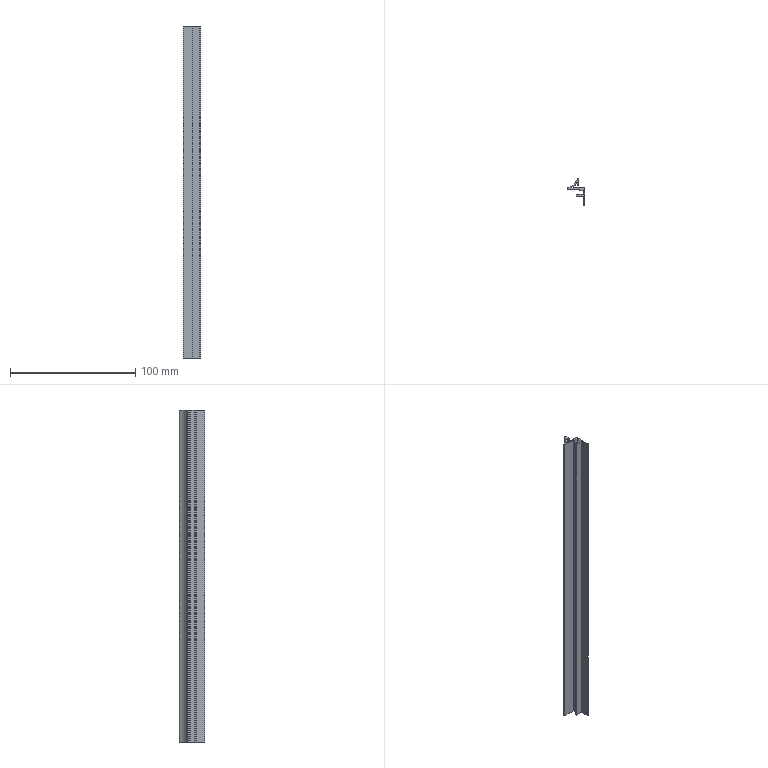Part | SolidWorks | features MoveFace 2, BaseBody 1, ICE 1 | 1 solid | 27 faces | box 14 x 20.3 x 265 mm | volume 13493 mm3 | plane 20 | cylinder 7 | commonest cylinder face diameters 0.387 x2 0.8 x2 0.4 x1 20 x1 22 x1
STEP:
#1=CARTESIAN_POINT('',(-5.304,-0.625,320.));
#2=VERTEX_POINT('',#1);
#3=CARTESIAN_POINT('',(-5.449,-0.8125,320.));
#4=VERTEX_POINT('',#3);
#5=CARTESIAN_POINT('',(-5.255,-0.8125,320.));
#6=DIRECTION('',(0.,0.,1.));
#7=DIRECTION('',(-1.,0.,0.));
#8=AXIS2_PLACEMENT_3D('',#5,#6,#7);
#9=CIRCLE('',#8,0.1937);
#10=EDGE_CURVE('',#2,#4,#9,.T.);
#11=ORIENTED_EDGE('',*,*,#10,.T.);
#12=CARTESIAN_POINT('',(-5.449,-0.8125,55.));
#13=VERTEX_POINT('',#12);
#14=CARTESIAN_POINT('',(-5.449,-0.8125,230.));
#15=DIRECTION('',(0.,0.,-1.));
#16=VECTOR('',#15,1000.);
#17=LINE('',#14,#16);
#18=EDGE_CURVE('',#4,#13,#17,.T.);
#19=ORIENTED_EDGE('',*,*,#18,.T.);
#20=CARTESIAN_POINT('',(-5.304,-0.625,55.));
#21=VERTEX_POINT('',#20);
#22=CARTESIAN_POINT('',(-5.255,-0.8125,55.));
#23=DIRECTION('',(0.,0.,-1.));
#24=DIRECTION('',(1.,0.,0.));
#25=AXIS2_PLACEMENT_3D('',#22,#23,#24);
#26=CIRCLE('',#25,0.1937);
#27=EDGE_CURVE('',#13,#21,#26,.T.);
#28=ORIENTED_EDGE('',*,*,#27,.T.);
#29=CARTESIAN_POINT('',(-5.304,-0.625,230.));
#30=DIRECTION('',(0.,0.,-1.));
#31=VECTOR('',#30,1000.);
#32=LINE('',#29,#31);
#33=EDGE_CURVE('',#2,#21,#32,.T.);
#34=ORIENTED_EDGE('',*,*,#33,.F.);
#35=EDGE_LOOP('',(#11,#19,#28,#34));
#36=FACE_OUTER_BOUND('',#35,.T.);
#37=CARTESIAN_POINT('',(-5.255,-0.8125,230.));
#38=DIRECTION('',(0.,0.,-1.));
#39=DIRECTION('',(-1.,0.,0.));
#40=AXIS2_PLACEMENT_3D('',#37,#38,#39);
#41=CYLINDRICAL_SURFACE('',#40,0.1937);
#42=ADVANCED_FACE('',(#36),#41,.F.);
#43=CARTESIAN_POINT('',(5.,-1.,55.));
#44=VERTEX_POINT('',#43);
#45=CARTESIAN_POINT('',(5.,-14.3,55.));
#46=VERTEX_POINT('',#45);
#47=CARTESIAN_POINT('',(5.,29.623,55.));
#48=DIRECTION('',(0.,-1.,0.));
#49=VECTOR('',#48,1000.);
#50=LINE('',#47,#49);
#51=EDGE_CURVE('',#44,#46,#50,.T.);
#52=ORIENTED_EDGE('',*,*,#51,.F.);
#53=CARTESIAN_POINT('',(5.,-1.,320.));
#54=VERTEX_POINT('',#53);
#55=CARTESIAN_POINT('',(5.,-1.,230.));
#56=DIRECTION('',(0.,0.,-1.));
#57=VECTOR('',#56,1000.);
#58=LINE('',#55,#57);
#59=EDGE_CURVE('',#54,#44,#58,.T.);
#60=ORIENTED_EDGE('',*,*,#59,.F.);
#61=CARTESIAN_POINT('',(5.,-14.3,320.));
#62=VERTEX_POINT('',#61);
#63=CARTESIAN_POINT('',(5.,29.623,320.));
#64=DIRECTION('',(0.,1.,0.));
#65=VECTOR('',#64,1000.);
#66=LINE('',#63,#65);
#67=EDGE_CURVE('',#62,#54,#66,.T.);
#68=ORIENTED_EDGE('',*,*,#67,.F.);
#69=CARTESIAN_POINT('',(5.,-14.3,230.));
#70=DIRECTION('',(0.,0.,1.));
#71=VECTOR('',#70,1000.);
#72=LINE('',#69,#71);
#73=EDGE_CURVE('',#46,#62,#72,.T.);
#74=ORIENTED_EDGE('',*,*,#73,.F.);
#75=EDGE_LOOP('',(#52,#60,#68,#74));
#76=FACE_OUTER_BOUND('',#75,.T.);
#77=CARTESIAN_POINT('',(5.,-14.3,230.));
#78=DIRECTION('',(-1.,0.,0.));
#79=DIRECTION('',(0.,0.,1.));
#80=AXIS2_PLACEMENT_3D('',#77,#78,#79);
#81=PLANE('',#80);
#82=ADVANCED_FACE('',(#76),#81,.F.);
#83=CARTESIAN_POINT('',(-9.,-2.,55.));
#84=VERTEX_POINT('',#83);
#85=CARTESIAN_POINT('',(-9.,-2.,320.));
#86=VERTEX_POINT('',#85);
#87=CARTESIAN_POINT('',(-9.,-2.,230.));
#88=DIRECTION('',(0.,0.,1.));
#89=VECTOR('',#88,1000.);
#90=LINE('',#87,#89);
#91=EDGE_CURVE('',#84,#86,#90,.T.);
#92=ORIENTED_EDGE('',*,*,#91,.F.);
#93=CARTESIAN_POINT('',(0.9,-2.,55.));
#94=VERTEX_POINT('',#93);
#95=CARTESIAN_POINT('',(5.,-2.,55.));
#96=DIRECTION('',(-1.,0.,0.));
#97=VECTOR('',#96,1000.);
#98=LINE('',#95,#97);
#99=EDGE_CURVE('',#94,#84,#98,.T.);
#100=ORIENTED_EDGE('',*,*,#99,.F.);
#101=CARTESIAN_POINT('',(0.9,-2.,320.));
#102=VERTEX_POINT('',#101);
#103=CARTESIAN_POINT('',(0.9,-2.,230.));
#104=DIRECTION('',(0.,0.,-1.));
#105=VECTOR('',#104,1000.);
#106=LINE('',#103,#105);
#107=EDGE_CURVE('',#102,#94,#106,.T.);
#108=ORIENTED_EDGE('',*,*,#107,.F.);
#109=CARTESIAN_POINT('',(5.,-2.,320.));
#110=DIRECTION('',(1.,0.,0.));
#111=VECTOR('',#110,1000.);
#112=LINE('',#109,#111);
#113=EDGE_CURVE('',#86,#102,#112,.T.);
#114=ORIENTED_EDGE('',*,*,#113,.F.);
#115=EDGE_LOOP('',(#92,#100,#108,#114));
#116=FACE_OUTER_BOUND('',#115,.T.);
#117=CARTESIAN_POINT('',(-9.,-2.,230.));
#118=DIRECTION('',(0.,1.,0.));
#119=DIRECTION('',(0.,0.,1.));
#120=AXIS2_PLACEMENT_3D('',#117,#118,#119);
#121=PLANE('',#120);
#122=ADVANCED_FACE('',(#116),#121,.F.);
#123=CARTESIAN_POINT('',(4.,-6.,320.));
#124=VERTEX_POINT('',#123);
#125=CARTESIAN_POINT('',(4.,-3.,320.));
#126=VERTEX_POINT('',#125);
#127=CARTESIAN_POINT('',(4.,-3.,320.));
#128=DIRECTION('',(0.,1.,0.));
#129=VECTOR('',#128,1000.);
#130=LINE('',#127,#129);
#131=EDGE_CURVE('',#124,#126,#130,.T.);
#132=ORIENTED_EDGE('',*,*,#131,.F.);
#133=CARTESIAN_POINT('',(1.,-6.,320.));
#134=VERTEX_POINT('',#133);
#135=CARTESIAN_POINT('',(4.,-6.,320.));
#136=DIRECTION('',(1.,0.,0.));
#137=VECTOR('',#136,1000.);
#138=LINE('',#135,#137);
#139=EDGE_CURVE('',#134,#124,#138,.T.);
#140=ORIENTED_EDGE('',*,*,#139,.F.);
#141=CARTESIAN_POINT('',(1.,-6.7,320.));
#142=VERTEX_POINT('',#141);
#143=CARTESIAN_POINT('',(1.,29.623,320.));
#144=DIRECTION('',(0.,-1.,0.));
#145=VECTOR('',#144,1000.);
#146=LINE('',#143,#145);
#147=EDGE_CURVE('',#134,#142,#146,.T.);
#148=ORIENTED_EDGE('',*,*,#147,.T.);
#149=CARTESIAN_POINT('',(-1.7,-6.7,320.));
#150=VERTEX_POINT('',#149);
#151=CARTESIAN_POINT('',(1.,-6.7,320.));
#152=DIRECTION('',(1.,0.,0.));
#153=VECTOR('',#152,1000.);
#154=LINE('',#151,#153);
#155=EDGE_CURVE('',#150,#142,#154,.T.);
#156=ORIENTED_EDGE('',*,*,#155,.F.);
#157=CARTESIAN_POINT('',(-1.7,-7.7,320.));
#158=VERTEX_POINT('',#157);
#159=CARTESIAN_POINT('',(-1.7,29.623,320.));
#160=DIRECTION('',(0.,-1.,0.));
#161=VECTOR('',#160,1000.);
#162=LINE('',#159,#161);
#163=EDGE_CURVE('',#150,#158,#162,.T.);
#164=ORIENTED_EDGE('',*,*,#163,.T.);
#165=CARTESIAN_POINT('',(4.,-7.7,320.));
#166=VERTEX_POINT('',#165);
#167=CARTESIAN_POINT('',(-1.7,-7.7,320.));
#168=DIRECTION('',(-1.,0.,0.));
#169=VECTOR('',#168,1000.);
#170=LINE('',#167,#169);
#171=EDGE_CURVE('',#166,#158,#170,.T.);
#172=ORIENTED_EDGE('',*,*,#171,.F.);
#173=CARTESIAN_POINT('',(4.,-14.3,320.));
#174=VERTEX_POINT('',#173);
#175=CARTESIAN_POINT('',(4.,-7.7,320.));
#176=DIRECTION('',(0.,1.,0.));
#177=VECTOR('',#176,1000.);
#178=LINE('',#175,#177);
#179=EDGE_CURVE('',#174,#166,#178,.T.);
#180=ORIENTED_EDGE('',*,*,#179,.F.);
#181=CARTESIAN_POINT('',(4.,-14.3,320.));
#182=DIRECTION('',(-1.,0.,0.));
#183=VECTOR('',#182,1000.);
#184=LINE('',#181,#183);
#185=EDGE_CURVE('',#62,#174,#184,.T.);
#186=ORIENTED_EDGE('',*,*,#185,.F.);
#187=ORIENTED_EDGE('',*,*,#67,.T.);
#188=CARTESIAN_POINT('',(-5.207,-1.,320.));
#189=VERTEX_POINT('',#188);
#190=CARTESIAN_POINT('',(5.,-1.,320.));
#191=DIRECTION('',(1.,0.,0.));
#192=VECTOR('',#191,1000.);
#193=LINE('',#190,#192);
#194=EDGE_CURVE('',#189,#54,#193,.T.);
#195=ORIENTED_EDGE('',*,*,#194,.F.);
#196=CARTESIAN_POINT('',(-5.255,-0.8125,320.));
#197=DIRECTION('',(0.,0.,1.));
#198=DIRECTION('',(-1.,0.,0.));
#199=AXIS2_PLACEMENT_3D('',#196,#197,#198);
#200=CIRCLE('',#199,0.1937);
#201=EDGE_CURVE('',#4,#189,#200,.T.);
#202=ORIENTED_EDGE('',*,*,#201,.F.);
#203=ORIENTED_EDGE('',*,*,#10,.F.);
#204=CARTESIAN_POINT('',(-1.368,3.063,320.));
#205=VERTEX_POINT('',#204);
#206=CARTESIAN_POINT('',(-10.628,9.,320.));
#207=DIRECTION('',(0.,0.,1.));
#208=DIRECTION('',(-1.,0.,0.));
#209=AXIS2_PLACEMENT_3D('',#206,#207,#208);
#210=CIRCLE('',#209,11.);
#211=EDGE_CURVE('',#2,#205,#210,.T.);
#212=ORIENTED_EDGE('',*,*,#211,.T.);
#213=CARTESIAN_POINT('',(-1.,2.955,320.));
#214=VERTEX_POINT('',#213);
#215=CARTESIAN_POINT('',(-1.2,2.955,320.));
#216=DIRECTION('',(0.,0.,1.));
#217=DIRECTION('',(-1.,0.,0.));
#218=AXIS2_PLACEMENT_3D('',#215,#216,#217);
#219=CIRCLE('',#218,0.2);
#220=EDGE_CURVE('',#214,#205,#219,.T.);
#221=ORIENTED_EDGE('',*,*,#220,.F.);
#222=CARTESIAN_POINT('',(-1.,1.5,320.));
#223=VERTEX_POINT('',#222);
#224=CARTESIAN_POINT('',(-1.,2.955,320.));
#225=DIRECTION('',(0.,1.,0.));
#226=VECTOR('',#225,1000.);
#227=LINE('',#224,#226);
#228=EDGE_CURVE('',#223,#214,#227,.T.);
#229=ORIENTED_EDGE('',*,*,#228,.F.);
#230=CARTESIAN_POINT('',(0.,1.5,320.));
#231=VERTEX_POINT('',#230);
#232=CARTESIAN_POINT('',(-1.,1.5,320.));
#233=DIRECTION('',(-1.,0.,0.));
#234=VECTOR('',#233,1000.);
#235=LINE('',#232,#234);
#236=EDGE_CURVE('',#231,#223,#235,.T.);
#237=ORIENTED_EDGE('',*,*,#236,.F.);
#238=CARTESIAN_POINT('',(0.,6.,320.));
#239=VERTEX_POINT('',#238);
#240=CARTESIAN_POINT('',(0.,1.5,320.));
#241=DIRECTION('',(0.,-1.,0.));
#242=VECTOR('',#241,1000.);
#243=LINE('',#240,#242);
#244=EDGE_CURVE('',#239,#231,#243,.T.);
#245=ORIENTED_EDGE('',*,*,#244,.F.);
#246=CARTESIAN_POINT('',(-0.8,6.,320.));
#247=VERTEX_POINT('',#246);
#248=CARTESIAN_POINT('',(0.,6.,320.));
#249=DIRECTION('',(1.,0.,0.));
#250=VECTOR('',#249,1000.);
#251=LINE('',#248,#250);
#252=EDGE_CURVE('',#247,#239,#251,.T.);
#253=ORIENTED_EDGE('',*,*,#252,.F.);
#254=CARTESIAN_POINT('',(-1.178,5.731,320.));
#255=VERTEX_POINT('',#254);
#256=CARTESIAN_POINT('',(-0.8,5.6,320.));
#257=DIRECTION('',(0.,0.,1.));
#258=DIRECTION('',(-1.,0.,0.));
#259=AXIS2_PLACEMENT_3D('',#256,#257,#258);
#260=CIRCLE('',#259,0.4);
#261=EDGE_CURVE('',#247,#255,#260,.T.);
#262=ORIENTED_EDGE('',*,*,#261,.T.);
#263=CARTESIAN_POINT('',(-8.678,-0.8077,320.));
#264=VERTEX_POINT('',#263);
#265=CARTESIAN_POINT('',(-10.628,9.,320.));
#266=DIRECTION('',(0.,0.,1.));
#267=DIRECTION('',(-1.,0.,0.));
#268=AXIS2_PLACEMENT_3D('',#265,#266,#267);
#269=CIRCLE('',#268,10.);
#270=EDGE_CURVE('',#264,#255,#269,.T.);
#271=ORIENTED_EDGE('',*,*,#270,.F.);
#272=CARTESIAN_POINT('',(-9.,-1.2,320.));
#273=VERTEX_POINT('',#272);
#274=CARTESIAN_POINT('',(-8.6,-1.2,320.));
#275=DIRECTION('',(0.,0.,1.));
#276=DIRECTION('',(-1.,0.,0.));
#277=AXIS2_PLACEMENT_3D('',#274,#275,#276);
#278=CIRCLE('',#277,0.4);
#279=EDGE_CURVE('',#264,#273,#278,.T.);
#280=ORIENTED_EDGE('',*,*,#279,.T.);
#281=CARTESIAN_POINT('',(-9.,29.623,320.));
#282=DIRECTION('',(0.,-1.,0.));
#283=VECTOR('',#282,1000.);
#284=LINE('',#281,#283);
#285=EDGE_CURVE('',#273,#86,#284,.T.);
#286=ORIENTED_EDGE('',*,*,#285,.T.);
#287=ORIENTED_EDGE('',*,*,#113,.T.);
#288=CARTESIAN_POINT('',(0.9,-3.,320.));
#289=VERTEX_POINT('',#288);
#290=CARTESIAN_POINT('',(0.9,-2.,320.));
#291=DIRECTION('',(0.,1.,0.));
#292=VECTOR('',#291,1000.);
#293=LINE('',#290,#292);
#294=EDGE_CURVE('',#289,#102,#293,.T.);
#295=ORIENTED_EDGE('',*,*,#294,.F.);
#296=CARTESIAN_POINT('',(0.9,-3.,320.));
#297=DIRECTION('',(-1.,0.,0.));
#298=VECTOR('',#297,1000.);
#299=LINE('',#296,#298);
#300=EDGE_CURVE('',#126,#289,#299,.T.);
#301=ORIENTED_EDGE('',*,*,#300,.F.);
#302=EDGE_LOOP('',(#132,#140,#148,#156,#164,#172,#180,#186,#187,#195,#202,#203,#212,#221,#229,#237,#245,#253,#262,#271,#280,#286,#287,#295,#301));
#303=FACE_OUTER_BOUND('',#302,.T.);
#304=CARTESIAN_POINT('',(5.,29.623,320.));
#305=DIRECTION('',(0.,0.,-1.));
#306=DIRECTION('',(-1.,0.,0.));
#307=AXIS2_PLACEMENT_3D('',#304,#305,#306);
#308=PLANE('',#307);
#309=ADVANCED_FACE('',(#303),#308,.F.);
#310=ORIENTED_EDGE('',*,*,#185,.T.);
#311=CARTESIAN_POINT('',(4.,-14.3,55.));
#312=VERTEX_POINT('',#311);
#313=CARTESIAN_POINT('',(4.,-14.3,230.));
#314=DIRECTION('',(0.,0.,1.));
#315=VECTOR('',#314,1000.);
#316=LINE('',#313,#315);
#317=EDGE_CURVE('',#312,#174,#316,.T.);
#318=ORIENTED_EDGE('',*,*,#317,.F.);
#319=CARTESIAN_POINT('',(5.,-14.3,55.));
#320=DIRECTION('',(-1.,0.,0.));
#321=VECTOR('',#320,1000.);
#322=LINE('',#319,#321);
#323=EDGE_CURVE('',#46,#312,#322,.T.);
#324=ORIENTED_EDGE('',*,*,#323,.F.);
#325=ORIENTED_EDGE('',*,*,#73,.T.);
#326=EDGE_LOOP('',(#310,#318,#324,#325));
#327=FACE_OUTER_BOUND('',#326,.T.);
#328=CARTESIAN_POINT('',(4.,-14.3,230.));
#329=DIRECTION('',(0.,1.,0.));
#330=DIRECTION('',(0.,0.,1.));
#331=AXIS2_PLACEMENT_3D('',#328,#329,#330);
#332=PLANE('',#331);
#333=ADVANCED_FACE('',(#327),#332,.F.);
#334=ORIENTED_EDGE('',*,*,#51,.T.);
#335=ORIENTED_EDGE('',*,*,#323,.T.);
#336=CARTESIAN_POINT('',(4.,-7.7,55.));
#337=VERTEX_POINT('',#336);
#338=CARTESIAN_POINT('',(4.,-7.7,55.));
#339=DIRECTION('',(0.,-1.,0.));
#340=VECTOR('',#339,1000.);
#341=LINE('',#338,#340);
#342=EDGE_CURVE('',#337,#312,#341,.T.);
#343=ORIENTED_EDGE('',*,*,#342,.F.);
#344=CARTESIAN_POINT('',(-1.7,-7.7,55.));
#345=VERTEX_POINT('',#344);
#346=CARTESIAN_POINT('',(-1.7,-7.7,55.));
#347=DIRECTION('',(1.,0.,0.));
#348=VECTOR('',#347,1000.);
#349=LINE('',#346,#348);
#350=EDGE_CURVE('',#345,#337,#349,.T.);
#351=ORIENTED_EDGE('',*,*,#350,.F.);
#352=CARTESIAN_POINT('',(-1.7,-6.7,55.));
#353=VERTEX_POINT('',#352);
#354=CARTESIAN_POINT('',(-1.7,29.623,55.));
#355=DIRECTION('',(0.,1.,0.));
#356=VECTOR('',#355,1000.);
#357=LINE('',#354,#356);
#358=EDGE_CURVE('',#345,#353,#357,.T.);
#359=ORIENTED_EDGE('',*,*,#358,.T.);
#360=CARTESIAN_POINT('',(1.,-6.7,55.));
#361=VERTEX_POINT('',#360);
#362=CARTESIAN_POINT('',(1.,-6.7,55.));
#363=DIRECTION('',(-1.,0.,0.));
#364=VECTOR('',#363,1000.);
#365=LINE('',#362,#364);
#366=EDGE_CURVE('',#361,#353,#365,.T.);
#367=ORIENTED_EDGE('',*,*,#366,.F.);
#368=CARTESIAN_POINT('',(1.,-6.,55.));
#369=VERTEX_POINT('',#368);
#370=CARTESIAN_POINT('',(1.,29.623,55.));
#371=DIRECTION('',(0.,1.,0.));
#372=VECTOR('',#371,1000.);
#373=LINE('',#370,#372);
#374=EDGE_CURVE('',#361,#369,#373,.T.);
#375=ORIENTED_EDGE('',*,*,#374,.T.);
#376=CARTESIAN_POINT('',(4.,-6.,55.));
#377=VERTEX_POINT('',#376);
#378=CARTESIAN_POINT('',(4.,-6.,55.));
#379=DIRECTION('',(-1.,0.,0.));
#380=VECTOR('',#379,1000.);
#381=LINE('',#378,#380);
#382=EDGE_CURVE('',#377,#369,#381,.T.);
#383=ORIENTED_EDGE('',*,*,#382,.F.);
#384=CARTESIAN_POINT('',(4.,-3.,55.));
#385=VERTEX_POINT('',#384);
#386=CARTESIAN_POINT('',(4.,-3.,55.));
#387=DIRECTION('',(0.,-1.,0.));
#388=VECTOR('',#387,1000.);
#389=LINE('',#386,#388);
#390=EDGE_CURVE('',#385,#377,#389,.T.);
#391=ORIENTED_EDGE('',*,*,#390,.F.);
#392=CARTESIAN_POINT('',(0.9,-3.,55.));
#393=VERTEX_POINT('',#392);
#394=CARTESIAN_POINT('',(0.9,-3.,55.));
#395=DIRECTION('',(1.,0.,0.));
#396=VECTOR('',#395,1000.);
#397=LINE('',#394,#396);
#398=EDGE_CURVE('',#393,#385,#397,.T.);
#399=ORIENTED_EDGE('',*,*,#398,.F.);
#400=CARTESIAN_POINT('',(0.9,-2.,55.));
#401=DIRECTION('',(0.,-1.,0.));
#402=VECTOR('',#401,1000.);
#403=LINE('',#400,#402);
#404=EDGE_CURVE('',#94,#393,#403,.T.);
#405=ORIENTED_EDGE('',*,*,#404,.F.);
#406=ORIENTED_EDGE('',*,*,#99,.T.);
#407=CARTESIAN_POINT('',(-9.,-1.2,55.));
#408=VERTEX_POINT('',#407);
#409=CARTESIAN_POINT('',(-9.,-1.2,55.));
#410=DIRECTION('',(0.,-1.,0.));
#411=VECTOR('',#410,1000.);
#412=LINE('',#409,#411);
#413=EDGE_CURVE('',#408,#84,#412,.T.);
#414=ORIENTED_EDGE('',*,*,#413,.F.);
#415=CARTESIAN_POINT('',(-8.678,-0.8077,55.));
#416=VERTEX_POINT('',#415);
#417=CARTESIAN_POINT('',(-8.6,-1.2,55.));
#418=DIRECTION('',(0.,0.,-1.));
#419=DIRECTION('',(1.,0.,0.));
#420=AXIS2_PLACEMENT_3D('',#417,#418,#419);
#421=CIRCLE('',#420,0.4);
#422=EDGE_CURVE('',#408,#416,#421,.T.);
#423=ORIENTED_EDGE('',*,*,#422,.T.);
#424=CARTESIAN_POINT('',(-1.178,5.731,55.));
#425=VERTEX_POINT('',#424);
#426=CARTESIAN_POINT('',(-10.628,9.,55.));
#427=DIRECTION('',(0.,0.,-1.));
#428=DIRECTION('',(1.,0.,0.));
#429=AXIS2_PLACEMENT_3D('',#426,#427,#428);
#430=CIRCLE('',#429,10.);
#431=EDGE_CURVE('',#425,#416,#430,.T.);
#432=ORIENTED_EDGE('',*,*,#431,.F.);
#433=CARTESIAN_POINT('',(-0.8,6.,55.));
#434=VERTEX_POINT('',#433);
#435=CARTESIAN_POINT('',(-0.8,5.6,55.));
#436=DIRECTION('',(0.,0.,-1.));
#437=DIRECTION('',(1.,0.,0.));
#438=AXIS2_PLACEMENT_3D('',#435,#436,#437);
#439=CIRCLE('',#438,0.4);
#440=EDGE_CURVE('',#425,#434,#439,.T.);
#441=ORIENTED_EDGE('',*,*,#440,.T.);
#442=CARTESIAN_POINT('',(0.,6.,55.));
#443=VERTEX_POINT('',#442);
#444=CARTESIAN_POINT('',(0.,6.,55.));
#445=DIRECTION('',(-1.,0.,0.));
#446=VECTOR('',#445,1000.);
#447=LINE('',#444,#446);
#448=EDGE_CURVE('',#443,#434,#447,.T.);
#449=ORIENTED_EDGE('',*,*,#448,.F.);
#450=CARTESIAN_POINT('',(0.,1.5,55.));
#451=VERTEX_POINT('',#450);
#452=CARTESIAN_POINT('',(0.,1.5,55.));
#453=DIRECTION('',(0.,1.,0.));
#454=VECTOR('',#453,1000.);
#455=LINE('',#452,#454);
#456=EDGE_CURVE('',#451,#443,#455,.T.);
#457=ORIENTED_EDGE('',*,*,#456,.F.);
#458=CARTESIAN_POINT('',(-1.,1.5,55.));
#459=VERTEX_POINT('',#458);
#460=CARTESIAN_POINT('',(-1.,1.5,55.));
#461=DIRECTION('',(1.,0.,0.));
#462=VECTOR('',#461,1000.);
#463=LINE('',#460,#462);
#464=EDGE_CURVE('',#459,#451,#463,.T.);
#465=ORIENTED_EDGE('',*,*,#464,.F.);
#466=CARTESIAN_POINT('',(-1.,2.955,55.));
#467=VERTEX_POINT('',#466);
#468=CARTESIAN_POINT('',(-1.,2.955,55.));
#469=DIRECTION('',(0.,-1.,0.));
#470=VECTOR('',#469,1000.);
#471=LINE('',#468,#470);
#472=EDGE_CURVE('',#467,#459,#471,.T.);
#473=ORIENTED_EDGE('',*,*,#472,.F.);
#474=CARTESIAN_POINT('',(-1.368,3.063,55.));
#475=VERTEX_POINT('',#474);
#476=CARTESIAN_POINT('',(-1.2,2.955,55.));
#477=DIRECTION('',(0.,0.,-1.));
#478=DIRECTION('',(1.,0.,0.));
#479=AXIS2_PLACEMENT_3D('',#476,#477,#478);
#480=CIRCLE('',#479,0.2);
#481=EDGE_CURVE('',#475,#467,#480,.T.);
#482=ORIENTED_EDGE('',*,*,#481,.F.);
#483=CARTESIAN_POINT('',(-10.628,9.,55.));
#484=DIRECTION('',(0.,0.,-1.));
#485=DIRECTION('',(1.,0.,0.));
#486=AXIS2_PLACEMENT_3D('',#483,#484,#485);
#487=CIRCLE('',#486,11.);
#488=EDGE_CURVE('',#475,#21,#487,.T.);
#489=ORIENTED_EDGE('',*,*,#488,.T.);
#490=ORIENTED_EDGE('',*,*,#27,.F.);
#491=CARTESIAN_POINT('',(-5.207,-1.,55.));
#492=VERTEX_POINT('',#491);
#493=CARTESIAN_POINT('',(-5.255,-0.8125,55.));
#494=DIRECTION('',(0.,0.,-1.));
#495=DIRECTION('',(1.,0.,0.));
#496=AXIS2_PLACEMENT_3D('',#493,#494,#495);
#497=CIRCLE('',#496,0.1937);
#498=EDGE_CURVE('',#492,#13,#497,.T.);
#499=ORIENTED_EDGE('',*,*,#498,.F.);
#500=CARTESIAN_POINT('',(5.,-1.,55.));
#501=DIRECTION('',(-1.,0.,0.));
#502=VECTOR('',#501,1000.);
#503=LINE('',#500,#502);
#504=EDGE_CURVE('',#44,#492,#503,.T.);
#505=ORIENTED_EDGE('',*,*,#504,.F.);
#506=EDGE_LOOP('',(#334,#335,#343,#351,#359,#367,#375,#383,#391,#399,#405,#406,#414,#423,#432,#441,#449,#457,#465,#473,#482,#489,#490,#499,#505));
#507=FACE_OUTER_BOUND('',#506,.T.);
#508=CARTESIAN_POINT('',(5.,29.623,55.));
#509=DIRECTION('',(0.,0.,1.));
#510=DIRECTION('',(1.,0.,0.));
#511=AXIS2_PLACEMENT_3D('',#508,#509,#510);
#512=PLANE('',#511);
#513=ADVANCED_FACE('',(#507),#512,.F.);
#514=ORIENTED_EDGE('',*,*,#59,.T.);
#515=ORIENTED_EDGE('',*,*,#504,.T.);
#516=CARTESIAN_POINT('',(-5.207,-1.,230.));
#517=DIRECTION('',(0.,0.,-1.));
#518=VECTOR('',#517,1000.);
#519=LINE('',#516,#518);
#520=EDGE_CURVE('',#189,#492,#519,.T.);
#521=ORIENTED_EDGE('',*,*,#520,.F.);
#522=ORIENTED_EDGE('',*,*,#194,.T.);
#523=EDGE_LOOP('',(#514,#515,#521,#522));
#524=FACE_OUTER_BOUND('',#523,.T.);
#525=CARTESIAN_POINT('',(5.,-1.,230.));
#526=DIRECTION('',(0.,-1.,0.));
#527=DIRECTION('',(0.,0.,-1.));
#528=AXIS2_PLACEMENT_3D('',#525,#526,#527);
#529=PLANE('',#528);
#530=ADVANCED_FACE('',(#524),#529,.F.);
#531=CARTESIAN_POINT('',(-9.,-1.2,230.));
#532=DIRECTION('',(0.,0.,1.));
#533=VECTOR('',#532,1000.);
#534=LINE('',#531,#533);
#535=EDGE_CURVE('',#408,#273,#534,.T.);
#536=ORIENTED_EDGE('',*,*,#535,.F.);
#537=ORIENTED_EDGE('',*,*,#413,.T.);
#538=ORIENTED_EDGE('',*,*,#91,.T.);
#539=ORIENTED_EDGE('',*,*,#285,.F.);
#540=EDGE_LOOP('',(#536,#537,#538,#539));
#541=FACE_OUTER_BOUND('',#540,.T.);
#542=CARTESIAN_POINT('',(-9.,-1.2,230.));
#543=DIRECTION('',(1.,0.,0.));
#544=DIRECTION('',(0.,0.,-1.));
#545=AXIS2_PLACEMENT_3D('',#542,#543,#544);
#546=PLANE('',#545);
#547=ADVANCED_FACE('',(#541),#546,.F.);
#548=ORIENTED_EDGE('',*,*,#294,.T.);
#549=ORIENTED_EDGE('',*,*,#107,.T.);
#550=ORIENTED_EDGE('',*,*,#404,.T.);
#551=CARTESIAN_POINT('',(0.9,-3.,230.));
#552=DIRECTION('',(0.,0.,-1.));
#553=VECTOR('',#552,1000.);
#554=LINE('',#551,#553);
#555=EDGE_CURVE('',#289,#393,#554,.T.);
#556=ORIENTED_EDGE('',*,*,#555,.F.);
#557=EDGE_LOOP('',(#548,#549,#550,#556));
#558=FACE_OUTER_BOUND('',#557,.T.);
#559=CARTESIAN_POINT('',(0.9,-2.,230.));
#560=DIRECTION('',(1.,0.,0.));
#561=DIRECTION('',(0.,0.,-1.));
#562=AXIS2_PLACEMENT_3D('',#559,#560,#561);
#563=PLANE('',#562);
#564=ADVANCED_FACE('',(#558),#563,.F.);
#565=ORIENTED_EDGE('',*,*,#300,.T.);
#566=ORIENTED_EDGE('',*,*,#555,.T.);
#567=ORIENTED_EDGE('',*,*,#398,.T.);
#568=CARTESIAN_POINT('',(4.,-3.,230.));
#569=DIRECTION('',(0.,0.,-1.));
#570=VECTOR('',#569,1000.);
#571=LINE('',#568,#570);
#572=EDGE_CURVE('',#126,#385,#571,.T.);
#573=ORIENTED_EDGE('',*,*,#572,.F.);
#574=EDGE_LOOP('',(#565,#566,#567,#573));
#575=FACE_OUTER_BOUND('',#574,.T.);
#576=CARTESIAN_POINT('',(0.9,-3.,230.));
#577=DIRECTION('',(0.,1.,0.));
#578=DIRECTION('',(0.,0.,1.));
#579=AXIS2_PLACEMENT_3D('',#576,#577,#578);
#580=PLANE('',#579);
#581=ADVANCED_FACE('',(#575),#580,.F.);
#582=ORIENTED_EDGE('',*,*,#131,.T.);
#583=ORIENTED_EDGE('',*,*,#572,.T.);
#584=ORIENTED_EDGE('',*,*,#390,.T.);
#585=CARTESIAN_POINT('',(4.,-6.,230.));
#586=DIRECTION('',(0.,0.,-1.));
#587=VECTOR('',#586,1000.);
#588=LINE('',#585,#587);
#589=EDGE_CURVE('',#124,#377,#588,.T.);
#590=ORIENTED_EDGE('',*,*,#589,.F.);
#591=EDGE_LOOP('',(#582,#583,#584,#590));
#592=FACE_OUTER_BOUND('',#591,.T.);
#593=CARTESIAN_POINT('',(4.,-3.,230.));
#594=DIRECTION('',(1.,0.,0.));
#595=DIRECTION('',(0.,0.,-1.));
#596=AXIS2_PLACEMENT_3D('',#593,#594,#595);
#597=PLANE('',#596);
#598=ADVANCED_FACE('',(#592),#597,.F.);
#599=ORIENTED_EDGE('',*,*,#139,.T.);
#600=ORIENTED_EDGE('',*,*,#589,.T.);
#601=ORIENTED_EDGE('',*,*,#382,.T.);
#602=CARTESIAN_POINT('',(1.,-6.,230.));
#603=DIRECTION('',(0.,0.,-1.));
#604=VECTOR('',#603,1000.);
#605=LINE('',#602,#604);
#606=EDGE_CURVE('',#134,#369,#605,.T.);
#607=ORIENTED_EDGE('',*,*,#606,.F.);
#608=EDGE_LOOP('',(#599,#600,#601,#607));
#609=FACE_OUTER_BOUND('',#608,.T.);
#610=CARTESIAN_POINT('',(4.,-6.,230.));
#611=DIRECTION('',(0.,-1.,0.));
#612=DIRECTION('',(0.,0.,-1.));
#613=AXIS2_PLACEMENT_3D('',#610,#611,#612);
#614=PLANE('',#613);
#615=ADVANCED_FACE('',(#609),#614,.F.);
#616=ORIENTED_EDGE('',*,*,#155,.T.);
#617=CARTESIAN_POINT('',(1.,-6.7,230.));
#618=DIRECTION('',(0.,0.,1.));
#619=VECTOR('',#618,1000.);
#620=LINE('',#617,#619);
#621=EDGE_CURVE('',#361,#142,#620,.T.);
#622=ORIENTED_EDGE('',*,*,#621,.F.);
#623=ORIENTED_EDGE('',*,*,#366,.T.);
#624=CARTESIAN_POINT('',(-1.7,-6.7,230.));
#625=DIRECTION('',(0.,0.,-1.));
#626=VECTOR('',#625,1000.);
#627=LINE('',#624,#626);
#628=EDGE_CURVE('',#150,#353,#627,.T.);
#629=ORIENTED_EDGE('',*,*,#628,.F.);
#630=EDGE_LOOP('',(#616,#622,#623,#629));
#631=FACE_OUTER_BOUND('',#630,.T.);
#632=CARTESIAN_POINT('',(1.,-6.7,230.));
#633=DIRECTION('',(0.,-1.,0.));
#634=DIRECTION('',(0.,0.,-1.));
#635=AXIS2_PLACEMENT_3D('',#632,#633,#634);
#636=PLANE('',#635);
#637=ADVANCED_FACE('',(#631),#636,.F.);
#638=ORIENTED_EDGE('',*,*,#171,.T.);
#639=CARTESIAN_POINT('',(-1.7,-7.7,230.));
#640=DIRECTION('',(0.,0.,1.));
#641=VECTOR('',#640,1000.);
#642=LINE('',#639,#641);
#643=EDGE_CURVE('',#345,#158,#642,.T.);
#644=ORIENTED_EDGE('',*,*,#643,.F.);
#645=ORIENTED_EDGE('',*,*,#350,.T.);
#646=CARTESIAN_POINT('',(4.,-7.7,230.));
#647=DIRECTION('',(0.,0.,-1.));
#648=VECTOR('',#647,1000.);
#649=LINE('',#646,#648);
#650=EDGE_CURVE('',#166,#337,#649,.T.);
#651=ORIENTED_EDGE('',*,*,#650,.F.);
#652=EDGE_LOOP('',(#638,#644,#645,#651));
#653=FACE_OUTER_BOUND('',#652,.T.);
#654=CARTESIAN_POINT('',(-1.7,-7.7,230.));
#655=DIRECTION('',(0.,1.,0.));
#656=DIRECTION('',(0.,0.,1.));
#657=AXIS2_PLACEMENT_3D('',#654,#655,#656);
#658=PLANE('',#657);
#659=ADVANCED_FACE('',(#653),#658,.F.);
#660=ORIENTED_EDGE('',*,*,#179,.T.);
#661=ORIENTED_EDGE('',*,*,#650,.T.);
#662=ORIENTED_EDGE('',*,*,#342,.T.);
#663=ORIENTED_EDGE('',*,*,#317,.T.);
#664=EDGE_LOOP('',(#660,#661,#662,#663));
#665=FACE_OUTER_BOUND('',#664,.T.);
#666=CARTESIAN_POINT('',(4.,-7.7,230.));
#667=DIRECTION('',(1.,0.,0.));
#668=DIRECTION('',(0.,0.,-1.));
#669=AXIS2_PLACEMENT_3D('',#666,#667,#668);
#670=PLANE('',#669);
#671=ADVANCED_FACE('',(#665),#670,.F.);
#672=ORIENTED_EDGE('',*,*,#18,.F.);
#673=ORIENTED_EDGE('',*,*,#201,.T.);
#674=ORIENTED_EDGE('',*,*,#520,.T.);
#675=ORIENTED_EDGE('',*,*,#498,.T.);
#676=EDGE_LOOP('',(#672,#673,#674,#675));
#677=FACE_OUTER_BOUND('',#676,.T.);
#678=CARTESIAN_POINT('',(-5.255,-0.8125,230.));
#679=DIRECTION('',(0.,0.,-1.));
#680=DIRECTION('',(-1.,0.,0.));
#681=AXIS2_PLACEMENT_3D('',#678,#679,#680);
#682=CYLINDRICAL_SURFACE('',#681,0.1937);
#683=ADVANCED_FACE('',(#677),#682,.F.);
#684=CARTESIAN_POINT('',(-1.,2.955,230.));
#685=DIRECTION('',(0.,0.,1.));
#686=VECTOR('',#685,1000.);
#687=LINE('',#684,#686);
#688=EDGE_CURVE('',#467,#214,#687,.T.);
#689=ORIENTED_EDGE('',*,*,#688,.F.);
#690=ORIENTED_EDGE('',*,*,#472,.T.);
#691=CARTESIAN_POINT('',(-1.,1.5,230.));
#692=DIRECTION('',(0.,0.,-1.));
#693=VECTOR('',#692,1000.);
#694=LINE('',#691,#693);
#695=EDGE_CURVE('',#223,#459,#694,.T.);
#696=ORIENTED_EDGE('',*,*,#695,.F.);
#697=ORIENTED_EDGE('',*,*,#228,.T.);
#698=EDGE_LOOP('',(#689,#690,#696,#697));
#699=FACE_OUTER_BOUND('',#698,.T.);
#700=CARTESIAN_POINT('',(-1.,2.955,230.));
#701=DIRECTION('',(1.,0.,0.));
#702=DIRECTION('',(0.,0.,-1.));
#703=AXIS2_PLACEMENT_3D('',#700,#701,#702);
#704=PLANE('',#703);
#705=ADVANCED_FACE('',(#699),#704,.F.);
#706=ORIENTED_EDGE('',*,*,#488,.F.);
#707=CARTESIAN_POINT('',(-1.368,3.063,230.));
#708=DIRECTION('',(0.,0.,1.));
#709=VECTOR('',#708,1000.);
#710=LINE('',#707,#709);
#711=EDGE_CURVE('',#475,#205,#710,.T.);
#712=ORIENTED_EDGE('',*,*,#711,.T.);
#713=ORIENTED_EDGE('',*,*,#211,.F.);
#714=ORIENTED_EDGE('',*,*,#33,.T.);
#715=EDGE_LOOP('',(#706,#712,#713,#714));
#716=FACE_OUTER_BOUND('',#715,.T.);
#717=CARTESIAN_POINT('',(-10.628,9.,230.));
#718=DIRECTION('',(0.,0.,-1.));
#719=DIRECTION('',(-1.,0.,0.));
#720=AXIS2_PLACEMENT_3D('',#717,#718,#719);
#721=CYLINDRICAL_SURFACE('',#720,11.);
#722=ADVANCED_FACE('',(#716),#721,.T.);
#723=CARTESIAN_POINT('',(-1.178,5.731,230.));
#724=DIRECTION('',(0.,0.,1.));
#725=VECTOR('',#724,1000.);
#726=LINE('',#723,#725);
#727=EDGE_CURVE('',#425,#255,#726,.T.);
#728=ORIENTED_EDGE('',*,*,#727,.F.);
#729=ORIENTED_EDGE('',*,*,#431,.T.);
#730=CARTESIAN_POINT('',(-8.678,-0.8077,230.));
#731=DIRECTION('',(0.,0.,-1.));
#732=VECTOR('',#731,1000.);
#733=LINE('',#730,#732);
#734=EDGE_CURVE('',#264,#416,#733,.T.);
#735=ORIENTED_EDGE('',*,*,#734,.F.);
#736=ORIENTED_EDGE('',*,*,#270,.T.);
#737=EDGE_LOOP('',(#728,#729,#735,#736));
#738=FACE_OUTER_BOUND('',#737,.T.);
#739=CARTESIAN_POINT('',(-10.628,9.,230.));
#740=DIRECTION('',(0.,0.,-1.));
#741=DIRECTION('',(-1.,0.,0.));
#742=AXIS2_PLACEMENT_3D('',#739,#740,#741);
#743=CYLINDRICAL_SURFACE('',#742,10.);
#744=ADVANCED_FACE('',(#738),#743,.F.);
#745=CARTESIAN_POINT('',(0.,1.5,230.));
#746=DIRECTION('',(0.,0.,1.));
#747=VECTOR('',#746,1000.);
#748=LINE('',#745,#747);
#749=EDGE_CURVE('',#451,#231,#748,.T.);
#750=ORIENTED_EDGE('',*,*,#749,.F.);
#751=ORIENTED_EDGE('',*,*,#456,.T.);
#752=CARTESIAN_POINT('',(0.,6.,230.));
#753=DIRECTION('',(0.,0.,-1.));
#754=VECTOR('',#753,1000.);
#755=LINE('',#752,#754);
#756=EDGE_CURVE('',#239,#443,#755,.T.);
#757=ORIENTED_EDGE('',*,*,#756,.F.);
#758=ORIENTED_EDGE('',*,*,#244,.T.);
#759=EDGE_LOOP('',(#750,#751,#757,#758));
#760=FACE_OUTER_BOUND('',#759,.T.);
#761=CARTESIAN_POINT('',(0.,1.5,230.));
#762=DIRECTION('',(-1.,0.,0.));
#763=DIRECTION('',(0.,0.,1.));
#764=AXIS2_PLACEMENT_3D('',#761,#762,#763);
#765=PLANE('',#764);
#766=ADVANCED_FACE('',(#760),#765,.F.);
#767=ORIENTED_EDGE('',*,*,#422,.F.);
#768=ORIENTED_EDGE('',*,*,#535,.T.);
#769=ORIENTED_EDGE('',*,*,#279,.F.);
#770=ORIENTED_EDGE('',*,*,#734,.T.);
#771=EDGE_LOOP('',(#767,#768,#769,#770));
#772=FACE_OUTER_BOUND('',#771,.T.);
#773=CARTESIAN_POINT('',(-8.6,-1.2,230.));
#774=DIRECTION('',(0.,0.,-1.));
#775=DIRECTION('',(-1.,0.,0.));
#776=AXIS2_PLACEMENT_3D('',#773,#774,#775);
#777=CYLINDRICAL_SURFACE('',#776,0.4);
#778=ADVANCED_FACE('',(#772),#777,.T.);
#779=ORIENTED_EDGE('',*,*,#147,.F.);
#780=ORIENTED_EDGE('',*,*,#606,.T.);
#781=ORIENTED_EDGE('',*,*,#374,.F.);
#782=ORIENTED_EDGE('',*,*,#621,.T.);
#783=EDGE_LOOP('',(#779,#780,#781,#782));
#784=FACE_OUTER_BOUND('',#783,.T.);
#785=CARTESIAN_POINT('',(1.,-6.,230.));
#786=DIRECTION('',(1.,0.,0.));
#787=DIRECTION('',(0.,0.,-1.));
#788=AXIS2_PLACEMENT_3D('',#785,#786,#787);
#789=PLANE('',#788);
#790=ADVANCED_FACE('',(#784),#789,.F.);
#791=ORIENTED_EDGE('',*,*,#163,.F.);
#792=ORIENTED_EDGE('',*,*,#628,.T.);
#793=ORIENTED_EDGE('',*,*,#358,.F.);
#794=ORIENTED_EDGE('',*,*,#643,.T.);
#795=EDGE_LOOP('',(#791,#792,#793,#794));
#796=FACE_OUTER_BOUND('',#795,.T.);
#797=CARTESIAN_POINT('',(-1.7,-6.7,230.));
#798=DIRECTION('',(1.,0.,0.));
#799=DIRECTION('',(0.,0.,-1.));
#800=AXIS2_PLACEMENT_3D('',#797,#798,#799);
#801=PLANE('',#800);
#802=ADVANCED_FACE('',(#796),#801,.F.);
#803=ORIENTED_EDGE('',*,*,#711,.F.);
#804=ORIENTED_EDGE('',*,*,#481,.T.);
#805=ORIENTED_EDGE('',*,*,#688,.T.);
#806=ORIENTED_EDGE('',*,*,#220,.T.);
#807=EDGE_LOOP('',(#803,#804,#805,#806));
#808=FACE_OUTER_BOUND('',#807,.T.);
#809=CARTESIAN_POINT('',(-1.2,2.955,230.));
#810=DIRECTION('',(0.,0.,-1.));
#811=DIRECTION('',(-1.,0.,0.));
#812=AXIS2_PLACEMENT_3D('',#809,#810,#811);
#813=CYLINDRICAL_SURFACE('',#812,0.2);
#814=ADVANCED_FACE('',(#808),#813,.F.);
#815=ORIENTED_EDGE('',*,*,#695,.T.);
#816=ORIENTED_EDGE('',*,*,#464,.T.);
#817=ORIENTED_EDGE('',*,*,#749,.T.);
#818=ORIENTED_EDGE('',*,*,#236,.T.);
#819=EDGE_LOOP('',(#815,#816,#817,#818));
#820=FACE_OUTER_BOUND('',#819,.T.);
#821=CARTESIAN_POINT('',(-1.,1.5,230.));
#822=DIRECTION('',(0.,1.,0.));
#823=DIRECTION('',(0.,0.,1.));
#824=AXIS2_PLACEMENT_3D('',#821,#822,#823);
#825=PLANE('',#824);
#826=ADVANCED_FACE('',(#820),#825,.F.);
#827=ORIENTED_EDGE('',*,*,#440,.F.);
#828=ORIENTED_EDGE('',*,*,#727,.T.);
#829=ORIENTED_EDGE('',*,*,#261,.F.);
#830=CARTESIAN_POINT('',(-0.8,6.,230.));
#831=DIRECTION('',(0.,0.,-1.));
#832=VECTOR('',#831,1000.);
#833=LINE('',#830,#832);
#834=EDGE_CURVE('',#247,#434,#833,.T.);
#835=ORIENTED_EDGE('',*,*,#834,.T.);
#836=EDGE_LOOP('',(#827,#828,#829,#835));
#837=FACE_OUTER_BOUND('',#836,.T.);
#838=CARTESIAN_POINT('',(-0.8,5.6,230.));
#839=DIRECTION('',(0.,0.,-1.));
#840=DIRECTION('',(-1.,0.,0.));
#841=AXIS2_PLACEMENT_3D('',#838,#839,#840);
#842=CYLINDRICAL_SURFACE('',#841,0.4);
#843=ADVANCED_FACE('',(#837),#842,.T.);
#844=ORIENTED_EDGE('',*,*,#756,.T.);
#845=ORIENTED_EDGE('',*,*,#448,.T.);
#846=ORIENTED_EDGE('',*,*,#834,.F.);
#847=ORIENTED_EDGE('',*,*,#252,.T.);
#848=EDGE_LOOP('',(#844,#845,#846,#847));
#849=FACE_OUTER_BOUND('',#848,.T.);
#850=CARTESIAN_POINT('',(0.,6.,230.));
#851=DIRECTION('',(0.,-1.,0.));
#852=DIRECTION('',(0.,0.,-1.));
#853=AXIS2_PLACEMENT_3D('',#850,#851,#852);
#854=PLANE('',#853);
#855=ADVANCED_FACE('',(#849),#854,.F.);
#856=CLOSED_SHELL('',(#42,#82,#122,#309,#333,#513,#530,#547,#564,#581,#598,#615,#637,#659,#671,#683,#705,#722,#744,#766,#778,#790,#802,#814,#826,#843,#855));
#857=MANIFOLD_SOLID_BREP('',#856);
#858=CARTESIAN_POINT('',(0.,0.,0.));
#859=DIRECTION('',(0.,0.,1.));
#860=DIRECTION('',(1.,0.,0.));
#861=AXIS2_PLACEMENT_3D('',#858,#859,#860);
#862=(LENGTH_UNIT()NAMED_UNIT(*)SI_UNIT(.MILLI.,.METRE.));
#863=UNCERTAINTY_MEASURE_WITH_UNIT(LENGTH_MEASURE(0.00001),#862,'','');
#864=(NAMED_UNIT(*)PLANE_ANGLE_UNIT()SI_UNIT($,.RADIAN.));
#865=(NAMED_UNIT(*)SI_UNIT($,.STERADIAN.)SOLID_ANGLE_UNIT());
#866=(GEOMETRIC_REPRESENTATION_CONTEXT(3)GLOBAL_UNCERTAINTY_ASSIGNED_CONTEXT((#863))GLOBAL_UNIT_ASSIGNED_CONTEXT((#862,#864,#865))REPRESENTATION_CONTEXT('',''));
#867=ADVANCED_BREP_SHAPE_REPRESENTATION('',(#857,#861),#866);